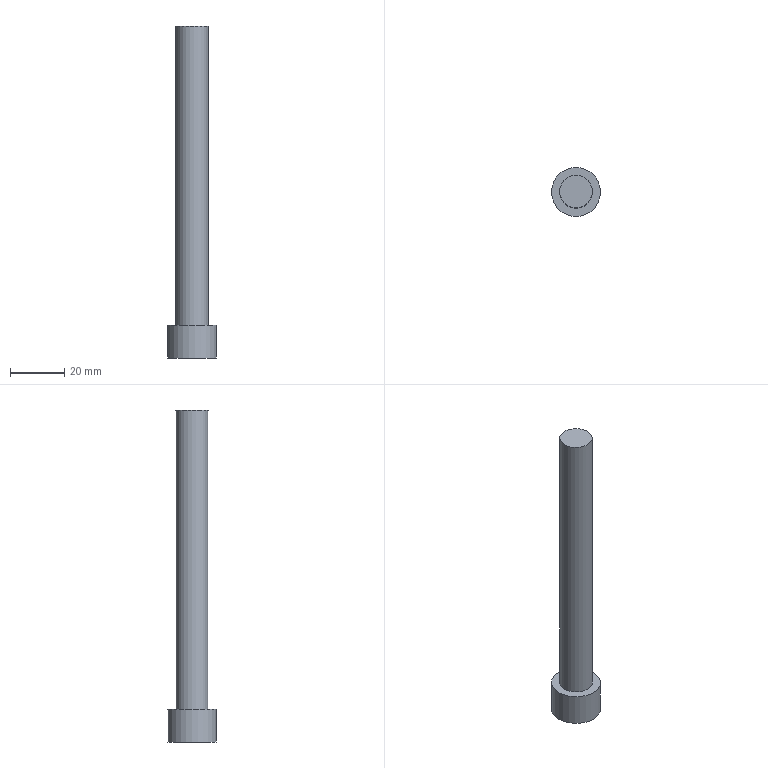Part | NX | features solid 2 | 1 solid | 12 faces | box 18 x 18 x 122 mm | volume 14920 mm3 | plane 10 | cylinder 2 | commonest cylinder face diameters 12 x1 18 x1
STEP:
#1=CARTESIAN_POINT('',(660.2,62.229,240.));
#2=VERTEX_POINT('',#1);
#3=CARTESIAN_POINT('',(665.,59.457,240.));
#4=VERTEX_POINT('',#3);
#5=CARTESIAN_POINT('',(662.6,60.843,240.));
#6=DIRECTION('',(0.866,-0.5,0.));
#7=VECTOR('',#6,1000.);
#8=LINE('',#5,#7);
#9=EDGE_CURVE('',#2,#4,#8,.T.);
#10=ORIENTED_EDGE('',*,*,#9,.T.);
#11=CARTESIAN_POINT('',(669.8,62.229,240.));
#12=VERTEX_POINT('',#11);
#13=CARTESIAN_POINT('',(667.4,60.843,240.));
#14=DIRECTION('',(0.866,0.5,0.));
#15=VECTOR('',#14,1000.);
#16=LINE('',#13,#15);
#17=EDGE_CURVE('',#4,#12,#16,.T.);
#18=ORIENTED_EDGE('',*,*,#17,.T.);
#19=CARTESIAN_POINT('',(669.8,67.771,240.));
#20=VERTEX_POINT('',#19);
#21=CARTESIAN_POINT('',(669.8,65.,240.));
#22=DIRECTION('',(0.,1.,0.));
#23=VECTOR('',#22,1000.);
#24=LINE('',#21,#23);
#25=EDGE_CURVE('',#12,#20,#24,.T.);
#26=ORIENTED_EDGE('',*,*,#25,.T.);
#27=CARTESIAN_POINT('',(665.,70.543,240.));
#28=VERTEX_POINT('',#27);
#29=CARTESIAN_POINT('',(667.4,69.157,240.));
#30=DIRECTION('',(-0.866,0.5,0.));
#31=VECTOR('',#30,1000.);
#32=LINE('',#29,#31);
#33=EDGE_CURVE('',#20,#28,#32,.T.);
#34=ORIENTED_EDGE('',*,*,#33,.T.);
#35=CARTESIAN_POINT('',(660.2,67.771,240.));
#36=VERTEX_POINT('',#35);
#37=CARTESIAN_POINT('',(662.6,69.157,240.));
#38=DIRECTION('',(-0.866,-0.5,0.));
#39=VECTOR('',#38,1000.);
#40=LINE('',#37,#39);
#41=EDGE_CURVE('',#28,#36,#40,.T.);
#42=ORIENTED_EDGE('',*,*,#41,.T.);
#43=CARTESIAN_POINT('',(660.2,65.,240.));
#44=DIRECTION('',(0.,-1.,0.));
#45=VECTOR('',#44,1000.);
#46=LINE('',#43,#45);
#47=EDGE_CURVE('',#36,#2,#46,.T.);
#48=ORIENTED_EDGE('',*,*,#47,.T.);
#49=EDGE_LOOP('',(#10,#18,#26,#34,#42,#48));
#50=FACE_BOUND('',#49,.T.);
#51=CARTESIAN_POINT('',(656.,65.,240.));
#52=VERTEX_POINT('',#51);
#53=CARTESIAN_POINT('',(665.,65.,240.));
#54=DIRECTION('',(0.,0.,-1.));
#55=DIRECTION('',(-1.,0.,0.));
#56=AXIS2_PLACEMENT_3D('',#53,#54,#55);
#57=CIRCLE('',#56,9.);
#58=EDGE_CURVE('',#52,#52,#57,.T.);
#59=ORIENTED_EDGE('',*,*,#58,.T.);
#60=EDGE_LOOP('',(#59));
#61=FACE_BOUND('',#60,.T.);
#62=CARTESIAN_POINT('',(665.,65.,240.));
#63=DIRECTION('',(0.,0.,-1.));
#64=DIRECTION('',(1.,0.,0.));
#65=AXIS2_PLACEMENT_3D('',#62,#63,#64);
#66=PLANE('',#65);
#67=ADVANCED_FACE('',(#50,#61),#66,.T.);
#68=CARTESIAN_POINT('',(659.,65.,252.));
#69=VERTEX_POINT('',#68);
#70=CARTESIAN_POINT('',(665.,65.,252.));
#71=DIRECTION('',(0.,0.,-1.));
#72=DIRECTION('',(-1.,0.,0.));
#73=AXIS2_PLACEMENT_3D('',#70,#71,#72);
#74=CIRCLE('',#73,6.);
#75=EDGE_CURVE('',#69,#69,#74,.T.);
#76=ORIENTED_EDGE('',*,*,#75,.T.);
#77=EDGE_LOOP('',(#76));
#78=FACE_BOUND('',#77,.T.);
#79=CARTESIAN_POINT('',(674.,65.,252.));
#80=VERTEX_POINT('',#79);
#81=CARTESIAN_POINT('',(665.,65.,252.));
#82=DIRECTION('',(0.,0.,1.));
#83=DIRECTION('',(1.,0.,0.));
#84=AXIS2_PLACEMENT_3D('',#81,#82,#83);
#85=CIRCLE('',#84,9.);
#86=EDGE_CURVE('',#80,#80,#85,.T.);
#87=ORIENTED_EDGE('',*,*,#86,.T.);
#88=EDGE_LOOP('',(#87));
#89=FACE_BOUND('',#88,.T.);
#90=CARTESIAN_POINT('',(665.,65.,252.));
#91=DIRECTION('',(0.,0.,1.));
#92=DIRECTION('',(-1.,0.,0.));
#93=AXIS2_PLACEMENT_3D('',#90,#91,#92);
#94=PLANE('',#93);
#95=ADVANCED_FACE('',(#78,#89),#94,.T.);
#96=ORIENTED_EDGE('',*,*,#58,.F.);
#97=EDGE_LOOP('',(#96));
#98=FACE_BOUND('',#97,.T.);
#99=ORIENTED_EDGE('',*,*,#86,.F.);
#100=EDGE_LOOP('',(#99));
#101=FACE_BOUND('',#100,.T.);
#102=CARTESIAN_POINT('',(665.,65.,252.));
#103=DIRECTION('',(0.,0.,-1.));
#104=DIRECTION('',(1.,0.,0.));
#105=AXIS2_PLACEMENT_3D('',#102,#103,#104);
#106=CYLINDRICAL_SURFACE('',#105,9.);
#107=ADVANCED_FACE('',(#98,#101),#106,.T.);
#108=ORIENTED_EDGE('',*,*,#9,.F.);
#109=CARTESIAN_POINT('',(660.2,62.229,247.2));
#110=VERTEX_POINT('',#109);
#111=CARTESIAN_POINT('',(660.2,62.229,247.2));
#112=DIRECTION('',(0.,0.,-1.));
#113=VECTOR('',#112,1000.);
#114=LINE('',#111,#113);
#115=EDGE_CURVE('',#110,#2,#114,.T.);
#116=ORIENTED_EDGE('',*,*,#115,.F.);
#117=CARTESIAN_POINT('',(665.,59.457,247.2));
#118=VERTEX_POINT('',#117);
#119=CARTESIAN_POINT('',(660.2,62.229,247.2));
#120=DIRECTION('',(0.866,-0.5,0.));
#121=VECTOR('',#120,1000.);
#122=LINE('',#119,#121);
#123=EDGE_CURVE('',#110,#118,#122,.T.);
#124=ORIENTED_EDGE('',*,*,#123,.T.);
#125=CARTESIAN_POINT('',(665.,59.457,247.2));
#126=DIRECTION('',(0.,0.,-1.));
#127=VECTOR('',#126,1000.);
#128=LINE('',#125,#127);
#129=EDGE_CURVE('',#118,#4,#128,.T.);
#130=ORIENTED_EDGE('',*,*,#129,.T.);
#131=EDGE_LOOP('',(#108,#116,#124,#130));
#132=FACE_BOUND('',#131,.T.);
#133=CARTESIAN_POINT('',(662.6,60.843,241.2));
#134=DIRECTION('',(-0.5,-0.866,0.));
#135=DIRECTION('',(0.866,-0.5,0.));
#136=AXIS2_PLACEMENT_3D('',#133,#134,#135);
#137=PLANE('',#136);
#138=ADVANCED_FACE('',(#132),#137,.F.);
#139=ORIENTED_EDGE('',*,*,#47,.F.);
#140=CARTESIAN_POINT('',(660.2,67.771,247.2));
#141=VERTEX_POINT('',#140);
#142=CARTESIAN_POINT('',(660.2,67.771,247.2));
#143=DIRECTION('',(0.,0.,-1.));
#144=VECTOR('',#143,1000.);
#145=LINE('',#142,#144);
#146=EDGE_CURVE('',#141,#36,#145,.T.);
#147=ORIENTED_EDGE('',*,*,#146,.F.);
#148=CARTESIAN_POINT('',(660.2,67.771,247.2));
#149=DIRECTION('',(0.,-1.,0.));
#150=VECTOR('',#149,1000.);
#151=LINE('',#148,#150);
#152=EDGE_CURVE('',#141,#110,#151,.T.);
#153=ORIENTED_EDGE('',*,*,#152,.T.);
#154=ORIENTED_EDGE('',*,*,#115,.T.);
#155=EDGE_LOOP('',(#139,#147,#153,#154));
#156=FACE_BOUND('',#155,.T.);
#157=CARTESIAN_POINT('',(660.2,65.,241.2));
#158=DIRECTION('',(-1.,0.,0.));
#159=DIRECTION('',(0.,0.,-1.));
#160=AXIS2_PLACEMENT_3D('',#157,#158,#159);
#161=PLANE('',#160);
#162=ADVANCED_FACE('',(#156),#161,.F.);
#163=ORIENTED_EDGE('',*,*,#41,.F.);
#164=CARTESIAN_POINT('',(665.,70.543,247.2));
#165=VERTEX_POINT('',#164);
#166=CARTESIAN_POINT('',(665.,70.543,247.2));
#167=DIRECTION('',(0.,0.,-1.));
#168=VECTOR('',#167,1000.);
#169=LINE('',#166,#168);
#170=EDGE_CURVE('',#165,#28,#169,.T.);
#171=ORIENTED_EDGE('',*,*,#170,.F.);
#172=CARTESIAN_POINT('',(665.,70.543,247.2));
#173=DIRECTION('',(-0.866,-0.5,0.));
#174=VECTOR('',#173,1000.);
#175=LINE('',#172,#174);
#176=EDGE_CURVE('',#165,#141,#175,.T.);
#177=ORIENTED_EDGE('',*,*,#176,.T.);
#178=ORIENTED_EDGE('',*,*,#146,.T.);
#179=EDGE_LOOP('',(#163,#171,#177,#178));
#180=FACE_BOUND('',#179,.T.);
#181=CARTESIAN_POINT('',(662.6,69.157,241.2));
#182=DIRECTION('',(-0.5,0.866,0.));
#183=DIRECTION('',(-0.866,-0.5,0.));
#184=AXIS2_PLACEMENT_3D('',#181,#182,#183);
#185=PLANE('',#184);
#186=ADVANCED_FACE('',(#180),#185,.F.);
#187=ORIENTED_EDGE('',*,*,#33,.F.);
#188=CARTESIAN_POINT('',(669.8,67.771,247.2));
#189=VERTEX_POINT('',#188);
#190=CARTESIAN_POINT('',(669.8,67.771,247.2));
#191=DIRECTION('',(0.,0.,-1.));
#192=VECTOR('',#191,1000.);
#193=LINE('',#190,#192);
#194=EDGE_CURVE('',#189,#20,#193,.T.);
#195=ORIENTED_EDGE('',*,*,#194,.F.);
#196=CARTESIAN_POINT('',(669.8,67.771,247.2));
#197=DIRECTION('',(-0.866,0.5,0.));
#198=VECTOR('',#197,1000.);
#199=LINE('',#196,#198);
#200=EDGE_CURVE('',#189,#165,#199,.T.);
#201=ORIENTED_EDGE('',*,*,#200,.T.);
#202=ORIENTED_EDGE('',*,*,#170,.T.);
#203=EDGE_LOOP('',(#187,#195,#201,#202));
#204=FACE_BOUND('',#203,.T.);
#205=CARTESIAN_POINT('',(667.4,69.157,241.2));
#206=DIRECTION('',(0.5,0.866,0.));
#207=DIRECTION('',(-0.866,0.5,0.));
#208=AXIS2_PLACEMENT_3D('',#205,#206,#207);
#209=PLANE('',#208);
#210=ADVANCED_FACE('',(#204),#209,.F.);
#211=ORIENTED_EDGE('',*,*,#25,.F.);
#212=CARTESIAN_POINT('',(669.8,62.229,247.2));
#213=VERTEX_POINT('',#212);
#214=CARTESIAN_POINT('',(669.8,62.229,247.2));
#215=DIRECTION('',(0.,0.,-1.));
#216=VECTOR('',#215,1000.);
#217=LINE('',#214,#216);
#218=EDGE_CURVE('',#213,#12,#217,.T.);
#219=ORIENTED_EDGE('',*,*,#218,.F.);
#220=CARTESIAN_POINT('',(669.8,62.229,247.2));
#221=DIRECTION('',(0.,1.,0.));
#222=VECTOR('',#221,1000.);
#223=LINE('',#220,#222);
#224=EDGE_CURVE('',#213,#189,#223,.T.);
#225=ORIENTED_EDGE('',*,*,#224,.T.);
#226=ORIENTED_EDGE('',*,*,#194,.T.);
#227=EDGE_LOOP('',(#211,#219,#225,#226));
#228=FACE_BOUND('',#227,.T.);
#229=CARTESIAN_POINT('',(669.8,65.,241.2));
#230=DIRECTION('',(1.,0.,0.));
#231=DIRECTION('',(0.,0.,1.));
#232=AXIS2_PLACEMENT_3D('',#229,#230,#231);
#233=PLANE('',#232);
#234=ADVANCED_FACE('',(#228),#233,.F.);
#235=ORIENTED_EDGE('',*,*,#17,.F.);
#236=ORIENTED_EDGE('',*,*,#129,.F.);
#237=CARTESIAN_POINT('',(665.,59.457,247.2));
#238=DIRECTION('',(0.866,0.5,0.));
#239=VECTOR('',#238,1000.);
#240=LINE('',#237,#239);
#241=EDGE_CURVE('',#118,#213,#240,.T.);
#242=ORIENTED_EDGE('',*,*,#241,.T.);
#243=ORIENTED_EDGE('',*,*,#218,.T.);
#244=EDGE_LOOP('',(#235,#236,#242,#243));
#245=FACE_BOUND('',#244,.T.);
#246=CARTESIAN_POINT('',(667.4,60.843,241.2));
#247=DIRECTION('',(0.5,-0.866,0.));
#248=DIRECTION('',(0.866,0.5,0.));
#249=AXIS2_PLACEMENT_3D('',#246,#247,#248);
#250=PLANE('',#249);
#251=ADVANCED_FACE('',(#245),#250,.F.);
#252=ORIENTED_EDGE('',*,*,#241,.F.);
#253=ORIENTED_EDGE('',*,*,#123,.F.);
#254=ORIENTED_EDGE('',*,*,#152,.F.);
#255=ORIENTED_EDGE('',*,*,#176,.F.);
#256=ORIENTED_EDGE('',*,*,#200,.F.);
#257=ORIENTED_EDGE('',*,*,#224,.F.);
#258=EDGE_LOOP('',(#252,#253,#254,#255,#256,#257));
#259=FACE_BOUND('',#258,.T.);
#260=CARTESIAN_POINT('',(665.,65.,247.2));
#261=DIRECTION('',(0.,0.,1.));
#262=DIRECTION('',(-1.,0.,0.));
#263=AXIS2_PLACEMENT_3D('',#260,#261,#262);
#264=PLANE('',#263);
#265=ADVANCED_FACE('',(#259),#264,.F.);
#266=CARTESIAN_POINT('',(671.,65.,362.));
#267=VERTEX_POINT('',#266);
#268=CARTESIAN_POINT('',(665.,65.,362.));
#269=DIRECTION('',(0.,0.,1.));
#270=DIRECTION('',(1.,0.,0.));
#271=AXIS2_PLACEMENT_3D('',#268,#269,#270);
#272=CIRCLE('',#271,6.);
#273=EDGE_CURVE('',#267,#267,#272,.T.);
#274=ORIENTED_EDGE('',*,*,#273,.T.);
#275=EDGE_LOOP('',(#274));
#276=FACE_BOUND('',#275,.T.);
#277=CARTESIAN_POINT('',(665.,65.,362.));
#278=DIRECTION('',(0.,0.,1.));
#279=DIRECTION('',(-1.,0.,0.));
#280=AXIS2_PLACEMENT_3D('',#277,#278,#279);
#281=PLANE('',#280);
#282=ADVANCED_FACE('',(#276),#281,.T.);
#283=ORIENTED_EDGE('',*,*,#273,.F.);
#284=EDGE_LOOP('',(#283));
#285=FACE_BOUND('',#284,.T.);
#286=ORIENTED_EDGE('',*,*,#75,.F.);
#287=EDGE_LOOP('',(#286));
#288=FACE_BOUND('',#287,.T.);
#289=CARTESIAN_POINT('',(665.,65.,252.));
#290=DIRECTION('',(0.,0.,1.));
#291=DIRECTION('',(-1.,0.,0.));
#292=AXIS2_PLACEMENT_3D('',#289,#290,#291);
#293=CYLINDRICAL_SURFACE('',#292,6.);
#294=ADVANCED_FACE('',(#285,#288),#293,.T.);
#295=CLOSED_SHELL('',(#67,#95,#107,#138,#162,#186,#210,#234,#251,#265,#282,#294));
#296=MANIFOLD_SOLID_BREP('',#295);
#297=(LENGTH_UNIT()NAMED_UNIT(*)SI_UNIT(.MILLI.,.METRE.));
#298=UNCERTAINTY_MEASURE_WITH_UNIT(LENGTH_MEASURE(0.00001),#297,'','');
#299=(NAMED_UNIT(*)PLANE_ANGLE_UNIT()SI_UNIT($,.RADIAN.));
#300=(NAMED_UNIT(*)SI_UNIT($,.STERADIAN.)SOLID_ANGLE_UNIT());
#301=(GEOMETRIC_REPRESENTATION_CONTEXT(3)GLOBAL_UNCERTAINTY_ASSIGNED_CONTEXT((#298))GLOBAL_UNIT_ASSIGNED_CONTEXT((#297,#299,#300))REPRESENTATION_CONTEXT('',''));
#302=ADVANCED_BREP_SHAPE_REPRESENTATION('',(#296),#301);